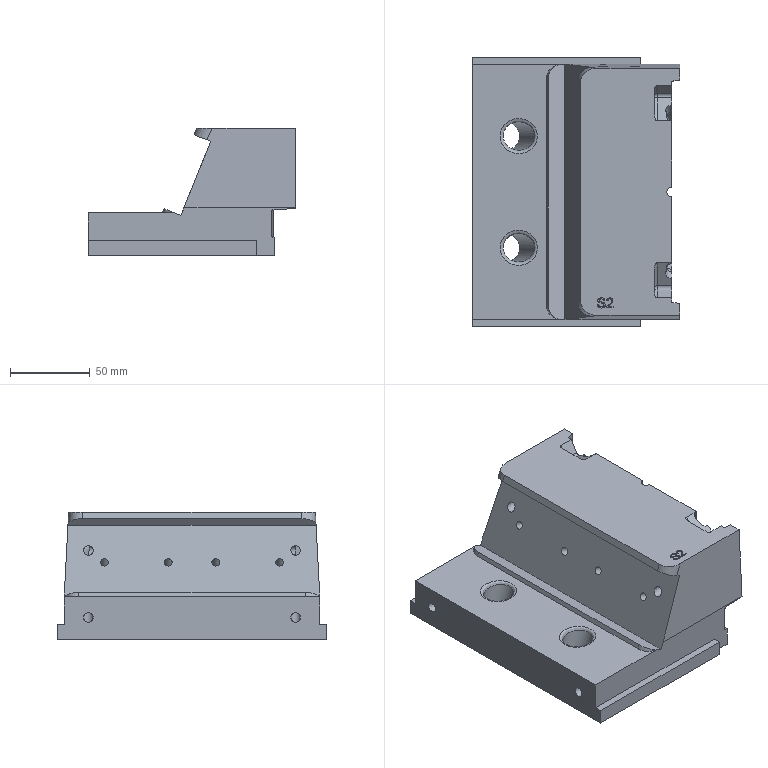Part | STEP file | lll_id86_x_t | 1 solid | 423 faces | box 130 x 169 x 80 mm | volume 855634 mm3 | plane 187 | cylinder 80 | spline 71 | other 61 | cone 10 | torus 10 | sphere 4 | commonest cylinder face diameters 6 x18 0.602 x14 2.008 x6 4 x6 18 x6 2 x4